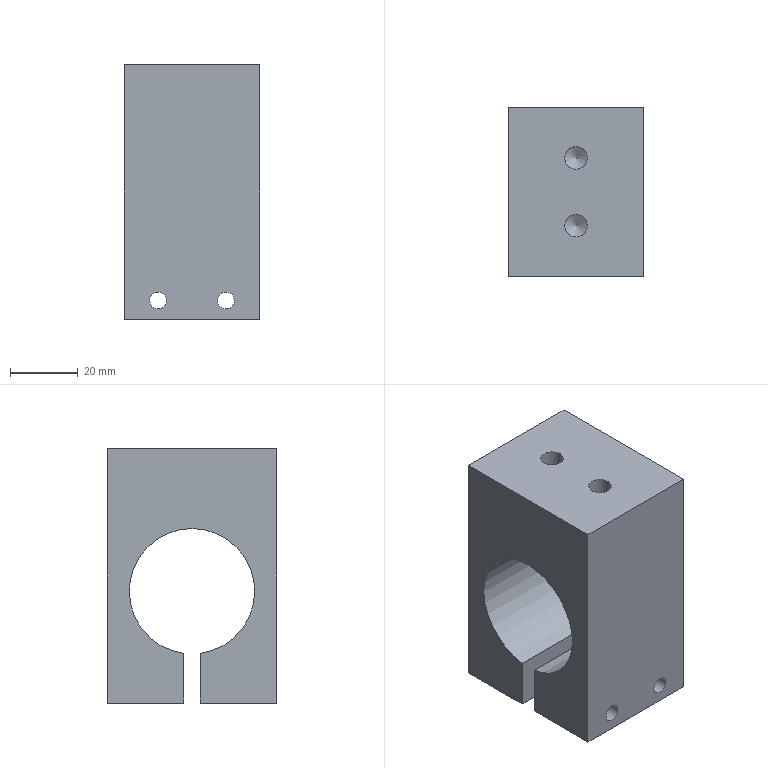Part | STEP file | SN10_010_003_SUPORTE | 1 solid | 18 faces | box 40 x 50 x 75 mm | volume 100062 mm3 | plane 9 | cylinder 7 | cone 2 | commonest cylinder face diameters 4.917 x2 6.647 x2 7 x2 37 x1
STEP:
#1=CARTESIAN_POINT('',(0.,0.,0.));
#2=DIRECTION('',(0.,0.,1.));
#3=DIRECTION('',(1.,0.,0.));
#4=AXIS2_PLACEMENT_3D('',#1,#2,#3);
#5=CARTESIAN_POINT('',(-7.842,117.5,231.679));
#6=VERTEX_POINT('',#5);
#7=CARTESIAN_POINT('',(-10.,117.5,230.5));
#8=DIRECTION('',(0.,1.,0.));
#9=DIRECTION('',(1.,0.,0.));
#10=AXIS2_PLACEMENT_3D('',#7,#8,#9);
#11=CIRCLE('',#10,2.458);
#12=CARTESIAN_POINT('',(-10.,117.4,230.5));
#13=DIRECTION('',(0.,-1.,0.));
#14=DIRECTION('',(0.8776,0.,0.4794));
#15=AXIS2_PLACEMENT_3D('',#12,#13,#14);
#16=CYLINDRICAL_SURFACE('',#15,2.458);
#17=CARTESIAN_POINT('',(12.066,-0.1));
#18=DIRECTION('',(-1.,0.));
#19=VECTOR('',#18,1.);
#20=LINE('',#17,#19);
#21=(GEOMETRIC_REPRESENTATION_CONTEXT(2)PARAMETRIC_REPRESENTATION_CONTEXT()REPRESENTATION_CONTEXT('',''));
#22=DEFINITIONAL_REPRESENTATION('',(#20),#21);
#23=PCURVE('',#16,#22);
#24=CARTESIAN_POINT('',(20.,117.5,239.67));
#25=DIRECTION('',(0.,1.,0.));
#26=DIRECTION('',(0.,0.,1.));
#27=AXIS2_PLACEMENT_3D('',#24,#25,#26);
#28=PLANE('',#27);
#29=CARTESIAN_POINT('',(-9.17,-30.));
#30=DIRECTION('',(0.,1.));
#31=AXIS2_PLACEMENT_2D('',#29,#30);
#32=CIRCLE('',#31,2.458);
#33=(GEOMETRIC_REPRESENTATION_CONTEXT(2)PARAMETRIC_REPRESENTATION_CONTEXT()REPRESENTATION_CONTEXT('',''));
#34=DEFINITIONAL_REPRESENTATION('',(#32),#33);
#35=PCURVE('',#28,#34);
#36=SURFACE_CURVE('',#11,(#23,#35),.PCURVE_S1.);
#37=EDGE_CURVE('',#6,#6,#36,.T.);
#38=ORIENTED_EDGE('',*,*,#37,.F.);
#39=CARTESIAN_POINT('',(-7.842,95.,231.679));
#40=VERTEX_POINT('',#39);
#41=CARTESIAN_POINT('',(-7.842,117.5,231.679));
#42=CARTESIAN_POINT('',(-7.842,95.,231.679));
#43=B_SPLINE_CURVE_WITH_KNOTS('',1,(#41,#42),.UNSPECIFIED.,.F.,.F.,(2,2),(-0.1,22.4),.PIECEWISE_BEZIER_KNOTS.);
#44=CARTESIAN_POINT('',(6.283,0.));
#45=DIRECTION('',(0.,1.));
#46=VECTOR('',#45,1.);
#47=LINE('',#44,#46);
#48=(GEOMETRIC_REPRESENTATION_CONTEXT(2)PARAMETRIC_REPRESENTATION_CONTEXT()REPRESENTATION_CONTEXT('',''));
#49=DEFINITIONAL_REPRESENTATION('',(#47),#48);
#50=PCURVE('',#16,#49);
#51=CARTESIAN_POINT('',(0.,0.));
#52=DIRECTION('',(0.,1.));
#53=VECTOR('',#52,1.);
#54=LINE('',#51,#53);
#55=(GEOMETRIC_REPRESENTATION_CONTEXT(2)PARAMETRIC_REPRESENTATION_CONTEXT()REPRESENTATION_CONTEXT('',''));
#56=DEFINITIONAL_REPRESENTATION('',(#54),#55);
#57=PCURVE('',#16,#56);
#58=SEAM_CURVE('',#43,(#50,#57),.PCURVE_S1.);
#59=EDGE_CURVE('',#6,#40,#58,.T.);
#60=ORIENTED_EDGE('',*,*,#59,.T.);
#61=CARTESIAN_POINT('',(-10.,95.,230.5));
#62=DIRECTION('',(0.,-1.,0.));
#63=DIRECTION('',(1.,0.,0.));
#64=AXIS2_PLACEMENT_3D('',#61,#62,#63);
#65=CIRCLE('',#64,2.458);
#66=CARTESIAN_POINT('',(-0.5,22.4));
#67=DIRECTION('',(1.,0.));
#68=VECTOR('',#67,1.);
#69=LINE('',#66,#68);
#70=(GEOMETRIC_REPRESENTATION_CONTEXT(2)PARAMETRIC_REPRESENTATION_CONTEXT()REPRESENTATION_CONTEXT('',''));
#71=DEFINITIONAL_REPRESENTATION('',(#69),#70);
#72=PCURVE('',#16,#71);
#73=CARTESIAN_POINT('',(0.,95.,300.));
#74=DIRECTION('',(0.,-1.,0.));
#75=DIRECTION('',(0.,0.,-1.));
#76=AXIS2_PLACEMENT_3D('',#73,#74,#75);
#77=PLANE('',#76);
#78=CARTESIAN_POINT('',(69.5,-10.));
#79=DIRECTION('',(0.,1.));
#80=AXIS2_PLACEMENT_2D('',#78,#79);
#81=CIRCLE('',#80,2.458);
#82=(GEOMETRIC_REPRESENTATION_CONTEXT(2)PARAMETRIC_REPRESENTATION_CONTEXT()REPRESENTATION_CONTEXT('',''));
#83=DEFINITIONAL_REPRESENTATION('',(#81),#82);
#84=PCURVE('',#77,#83);
#85=SURFACE_CURVE('',#65,(#72,#84),.PCURVE_S1.);
#86=EDGE_CURVE('',#40,#40,#85,.T.);
#87=ORIENTED_EDGE('',*,*,#86,.F.);
#88=ORIENTED_EDGE('',*,*,#59,.F.);
#89=EDGE_LOOP('',(#38,#60,#87,#88));
#90=FACE_BOUND('',#89,.F.);
#91=ADVANCED_FACE('',(#90),#16,.F.);
#92=CARTESIAN_POINT('',(20.,117.5,239.67));
#93=VERTEX_POINT('',#92);
#94=CARTESIAN_POINT('',(-20.,117.5,239.67));
#95=VERTEX_POINT('',#94);
#96=CARTESIAN_POINT('',(20.,117.5,239.67));
#97=DIRECTION('',(-1.,0.,0.));
#98=VECTOR('',#97,1.);
#99=LINE('',#96,#98);
#100=CARTESIAN_POINT('',(0.,0.));
#101=DIRECTION('',(0.,-1.));
#102=VECTOR('',#101,1.);
#103=LINE('',#100,#102);
#104=(GEOMETRIC_REPRESENTATION_CONTEXT(2)PARAMETRIC_REPRESENTATION_CONTEXT()REPRESENTATION_CONTEXT('',''));
#105=DEFINITIONAL_REPRESENTATION('',(#103),#104);
#106=PCURVE('',#28,#105);
#107=CARTESIAN_POINT('',(19.9,120.,258.));
#108=DIRECTION('',(-1.,0.,0.));
#109=DIRECTION('',(0.,0.8776,-0.4794));
#110=AXIS2_PLACEMENT_3D('',#107,#108,#109);
#111=CYLINDRICAL_SURFACE('',#110,18.5);
#112=CARTESIAN_POINT('',(1.206,-0.1));
#113=DIRECTION('',(0.,1.));
#114=VECTOR('',#113,1.);
#115=LINE('',#112,#114);
#116=(GEOMETRIC_REPRESENTATION_CONTEXT(2)PARAMETRIC_REPRESENTATION_CONTEXT()REPRESENTATION_CONTEXT('',''));
#117=DEFINITIONAL_REPRESENTATION('',(#115),#116);
#118=PCURVE('',#111,#117);
#119=SURFACE_CURVE('',#99,(#106,#118),.PCURVE_S1.);
#120=EDGE_CURVE('',#93,#95,#119,.T.);
#121=ORIENTED_EDGE('',*,*,#120,.F.);
#122=CARTESIAN_POINT('',(20.,117.5,225.));
#123=VERTEX_POINT('',#122);
#124=CARTESIAN_POINT('',(20.,117.5,239.67));
#125=DIRECTION('',(0.,0.,-1.));
#126=VECTOR('',#125,1.);
#127=LINE('',#124,#126);
#128=CARTESIAN_POINT('',(0.,0.));
#129=DIRECTION('',(-1.,0.));
#130=VECTOR('',#129,1.);
#131=LINE('',#128,#130);
#132=(GEOMETRIC_REPRESENTATION_CONTEXT(2)PARAMETRIC_REPRESENTATION_CONTEXT()REPRESENTATION_CONTEXT('',''));
#133=DEFINITIONAL_REPRESENTATION('',(#131),#132);
#134=PCURVE('',#28,#133);
#135=CARTESIAN_POINT('',(20.,120.,300.));
#136=DIRECTION('',(1.,0.,0.));
#137=DIRECTION('',(0.,0.,-1.));
#138=AXIS2_PLACEMENT_3D('',#135,#136,#137);
#139=PLANE('',#138);
#140=CARTESIAN_POINT('',(60.33,-2.5));
#141=DIRECTION('',(1.,0.));
#142=VECTOR('',#141,1.);
#143=LINE('',#140,#142);
#144=(GEOMETRIC_REPRESENTATION_CONTEXT(2)PARAMETRIC_REPRESENTATION_CONTEXT()REPRESENTATION_CONTEXT('',''));
#145=DEFINITIONAL_REPRESENTATION('',(#143),#144);
#146=PCURVE('',#139,#145);
#147=SURFACE_CURVE('',#127,(#134,#146),.PCURVE_S1.);
#148=EDGE_CURVE('',#93,#123,#147,.T.);
#149=ORIENTED_EDGE('',*,*,#148,.T.);
#150=CARTESIAN_POINT('',(-20.,117.5,225.));
#151=VERTEX_POINT('',#150);
#152=CARTESIAN_POINT('',(20.,117.5,225.));
#153=DIRECTION('',(-1.,0.,0.));
#154=VECTOR('',#153,1.);
#155=LINE('',#152,#154);
#156=CARTESIAN_POINT('',(-14.67,0.));
#157=DIRECTION('',(0.,-1.));
#158=VECTOR('',#157,1.);
#159=LINE('',#156,#158);
#160=(GEOMETRIC_REPRESENTATION_CONTEXT(2)PARAMETRIC_REPRESENTATION_CONTEXT()REPRESENTATION_CONTEXT('',''));
#161=DEFINITIONAL_REPRESENTATION('',(#159),#160);
#162=PCURVE('',#28,#161);
#163=CARTESIAN_POINT('',(0.,145.,225.));
#164=DIRECTION('',(0.,0.,1.));
#165=DIRECTION('',(1.,0.,0.));
#166=AXIS2_PLACEMENT_3D('',#163,#164,#165);
#167=PLANE('',#166);
#168=CARTESIAN_POINT('',(20.,-27.5));
#169=DIRECTION('',(-1.,0.));
#170=VECTOR('',#169,1.);
#171=LINE('',#168,#170);
#172=(GEOMETRIC_REPRESENTATION_CONTEXT(2)PARAMETRIC_REPRESENTATION_CONTEXT()REPRESENTATION_CONTEXT('',''));
#173=DEFINITIONAL_REPRESENTATION('',(#171),#172);
#174=PCURVE('',#167,#173);
#175=SURFACE_CURVE('',#155,(#162,#174),.PCURVE_S1.);
#176=EDGE_CURVE('',#123,#151,#175,.T.);
#177=ORIENTED_EDGE('',*,*,#176,.T.);
#178=CARTESIAN_POINT('',(-20.,117.5,225.));
#179=DIRECTION('',(0.,0.,1.));
#180=VECTOR('',#179,1.);
#181=LINE('',#178,#180);
#182=CARTESIAN_POINT('',(-14.67,-40.));
#183=DIRECTION('',(1.,0.));
#184=VECTOR('',#183,1.);
#185=LINE('',#182,#184);
#186=(GEOMETRIC_REPRESENTATION_CONTEXT(2)PARAMETRIC_REPRESENTATION_CONTEXT()REPRESENTATION_CONTEXT('',''));
#187=DEFINITIONAL_REPRESENTATION('',(#185),#186);
#188=PCURVE('',#28,#187);
#189=CARTESIAN_POINT('',(-20.,120.,300.));
#190=DIRECTION('',(1.,0.,0.));
#191=DIRECTION('',(0.,0.,-1.));
#192=AXIS2_PLACEMENT_3D('',#189,#190,#191);
#193=PLANE('',#192);
#194=CARTESIAN_POINT('',(75.,-2.5));
#195=DIRECTION('',(-1.,0.));
#196=VECTOR('',#195,1.);
#197=LINE('',#194,#196);
#198=(GEOMETRIC_REPRESENTATION_CONTEXT(2)PARAMETRIC_REPRESENTATION_CONTEXT()REPRESENTATION_CONTEXT('',''));
#199=DEFINITIONAL_REPRESENTATION('',(#197),#198);
#200=PCURVE('',#193,#199);
#201=SURFACE_CURVE('',#181,(#188,#200),.PCURVE_S1.);
#202=EDGE_CURVE('',#151,#95,#201,.T.);
#203=ORIENTED_EDGE('',*,*,#202,.T.);
#204=EDGE_LOOP('',(#121,#149,#177,#203));
#205=FACE_BOUND('',#204,.T.);
#206=ORIENTED_EDGE('',*,*,#37,.F.);
#207=EDGE_LOOP('',(#206));
#208=FACE_BOUND('',#207,.T.);
#209=CARTESIAN_POINT('',(12.158,117.5,231.679));
#210=VERTEX_POINT('',#209);
#211=CARTESIAN_POINT('',(10.,117.5,230.5));
#212=DIRECTION('',(0.,1.,0.));
#213=DIRECTION('',(1.,0.,0.));
#214=AXIS2_PLACEMENT_3D('',#211,#212,#213);
#215=CIRCLE('',#214,2.458);
#216=CARTESIAN_POINT('',(-9.17,-10.));
#217=DIRECTION('',(0.,1.));
#218=AXIS2_PLACEMENT_2D('',#216,#217);
#219=CIRCLE('',#218,2.458);
#220=(GEOMETRIC_REPRESENTATION_CONTEXT(2)PARAMETRIC_REPRESENTATION_CONTEXT()REPRESENTATION_CONTEXT('',''));
#221=DEFINITIONAL_REPRESENTATION('',(#219),#220);
#222=PCURVE('',#28,#221);
#223=CARTESIAN_POINT('',(10.,117.4,230.5));
#224=DIRECTION('',(0.,-1.,0.));
#225=DIRECTION('',(0.8776,0.,0.4794));
#226=AXIS2_PLACEMENT_3D('',#223,#224,#225);
#227=CYLINDRICAL_SURFACE('',#226,2.458);
#228=CARTESIAN_POINT('',(12.066,-0.1));
#229=DIRECTION('',(-1.,0.));
#230=VECTOR('',#229,1.);
#231=LINE('',#228,#230);
#232=(GEOMETRIC_REPRESENTATION_CONTEXT(2)PARAMETRIC_REPRESENTATION_CONTEXT()REPRESENTATION_CONTEXT('',''));
#233=DEFINITIONAL_REPRESENTATION('',(#231),#232);
#234=PCURVE('',#227,#233);
#235=SURFACE_CURVE('',#215,(#222,#234),.PCURVE_S1.);
#236=EDGE_CURVE('',#210,#210,#235,.T.);
#237=ORIENTED_EDGE('',*,*,#236,.F.);
#238=EDGE_LOOP('',(#237));
#239=FACE_BOUND('',#238,.T.);
#240=ADVANCED_FACE('',(#205,#208,#239),#28,.T.);
#241=CARTESIAN_POINT('',(-20.,95.,300.));
#242=VERTEX_POINT('',#241);
#243=CARTESIAN_POINT('',(20.,95.,300.));
#244=VERTEX_POINT('',#243);
#245=CARTESIAN_POINT('',(-20.,95.,300.));
#246=DIRECTION('',(1.,0.,0.));
#247=VECTOR('',#246,1.);
#248=LINE('',#245,#247);
#249=CARTESIAN_POINT('',(0.,-20.));
#250=DIRECTION('',(0.,1.));
#251=VECTOR('',#250,1.);
#252=LINE('',#249,#251);
#253=(GEOMETRIC_REPRESENTATION_CONTEXT(2)PARAMETRIC_REPRESENTATION_CONTEXT()REPRESENTATION_CONTEXT('',''));
#254=DEFINITIONAL_REPRESENTATION('',(#252),#253);
#255=PCURVE('',#77,#254);
#256=CARTESIAN_POINT('',(0.,95.,300.));
#257=DIRECTION('',(0.,0.,-1.));
#258=DIRECTION('',(-1.,0.,0.));
#259=AXIS2_PLACEMENT_3D('',#256,#257,#258);
#260=PLANE('',#259);
#261=CARTESIAN_POINT('',(20.,0.));
#262=DIRECTION('',(-1.,0.));
#263=VECTOR('',#262,1.);
#264=LINE('',#261,#263);
#265=(GEOMETRIC_REPRESENTATION_CONTEXT(2)PARAMETRIC_REPRESENTATION_CONTEXT()REPRESENTATION_CONTEXT('',''));
#266=DEFINITIONAL_REPRESENTATION('',(#264),#265);
#267=PCURVE('',#260,#266);
#268=SURFACE_CURVE('',#248,(#255,#267),.PCURVE_S1.);
#269=EDGE_CURVE('',#242,#244,#268,.T.);
#270=ORIENTED_EDGE('',*,*,#269,.F.);
#271=CARTESIAN_POINT('',(-20.,95.,225.));
#272=VERTEX_POINT('',#271);
#273=CARTESIAN_POINT('',(-20.,95.,300.));
#274=DIRECTION('',(0.,0.,-1.));
#275=VECTOR('',#274,1.);
#276=LINE('',#273,#275);
#277=CARTESIAN_POINT('',(0.,-20.));
#278=DIRECTION('',(1.,0.));
#279=VECTOR('',#278,1.);
#280=LINE('',#277,#279);
#281=(GEOMETRIC_REPRESENTATION_CONTEXT(2)PARAMETRIC_REPRESENTATION_CONTEXT()REPRESENTATION_CONTEXT('',''));
#282=DEFINITIONAL_REPRESENTATION('',(#280),#281);
#283=PCURVE('',#77,#282);
#284=CARTESIAN_POINT('',(0.,-25.));
#285=DIRECTION('',(1.,0.));
#286=VECTOR('',#285,1.);
#287=LINE('',#284,#286);
#288=(GEOMETRIC_REPRESENTATION_CONTEXT(2)PARAMETRIC_REPRESENTATION_CONTEXT()REPRESENTATION_CONTEXT('',''));
#289=DEFINITIONAL_REPRESENTATION('',(#287),#288);
#290=PCURVE('',#193,#289);
#291=SURFACE_CURVE('',#276,(#283,#290),.PCURVE_S1.);
#292=EDGE_CURVE('',#242,#272,#291,.T.);
#293=ORIENTED_EDGE('',*,*,#292,.T.);
#294=CARTESIAN_POINT('',(20.,95.,225.));
#295=VERTEX_POINT('',#294);
#296=CARTESIAN_POINT('',(-20.,95.,225.));
#297=DIRECTION('',(1.,0.,0.));
#298=VECTOR('',#297,1.);
#299=LINE('',#296,#298);
#300=CARTESIAN_POINT('',(75.,-20.));
#301=DIRECTION('',(0.,1.));
#302=VECTOR('',#301,1.);
#303=LINE('',#300,#302);
#304=(GEOMETRIC_REPRESENTATION_CONTEXT(2)PARAMETRIC_REPRESENTATION_CONTEXT()REPRESENTATION_CONTEXT('',''));
#305=DEFINITIONAL_REPRESENTATION('',(#303),#304);
#306=PCURVE('',#77,#305);
#307=CARTESIAN_POINT('',(-20.,-50.));
#308=DIRECTION('',(1.,0.));
#309=VECTOR('',#308,1.);
#310=LINE('',#307,#309);
#311=(GEOMETRIC_REPRESENTATION_CONTEXT(2)PARAMETRIC_REPRESENTATION_CONTEXT()REPRESENTATION_CONTEXT('',''));
#312=DEFINITIONAL_REPRESENTATION('',(#310),#311);
#313=PCURVE('',#167,#312);
#314=SURFACE_CURVE('',#299,(#306,#313),.PCURVE_S1.);
#315=EDGE_CURVE('',#272,#295,#314,.T.);
#316=ORIENTED_EDGE('',*,*,#315,.T.);
#317=CARTESIAN_POINT('',(20.,95.,300.));
#318=DIRECTION('',(0.,0.,-1.));
#319=VECTOR('',#318,1.);
#320=LINE('',#317,#319);
#321=CARTESIAN_POINT('',(0.,20.));
#322=DIRECTION('',(1.,0.));
#323=VECTOR('',#322,1.);
#324=LINE('',#321,#323);
#325=(GEOMETRIC_REPRESENTATION_CONTEXT(2)PARAMETRIC_REPRESENTATION_CONTEXT()REPRESENTATION_CONTEXT('',''));
#326=DEFINITIONAL_REPRESENTATION('',(#324),#325);
#327=PCURVE('',#77,#326);
#328=CARTESIAN_POINT('',(0.,-25.));
#329=DIRECTION('',(1.,0.));
#330=VECTOR('',#329,1.);
#331=LINE('',#328,#330);
#332=(GEOMETRIC_REPRESENTATION_CONTEXT(2)PARAMETRIC_REPRESENTATION_CONTEXT()REPRESENTATION_CONTEXT('',''));
#333=DEFINITIONAL_REPRESENTATION('',(#331),#332);
#334=PCURVE('',#139,#333);
#335=SURFACE_CURVE('',#320,(#327,#334),.PCURVE_S1.);
#336=EDGE_CURVE('',#244,#295,#335,.T.);
#337=ORIENTED_EDGE('',*,*,#336,.F.);
#338=EDGE_LOOP('',(#270,#293,#316,#337));
#339=FACE_BOUND('',#338,.T.);
#340=ORIENTED_EDGE('',*,*,#86,.F.);
#341=EDGE_LOOP('',(#340));
#342=FACE_BOUND('',#341,.T.);
#343=CARTESIAN_POINT('',(12.158,95.,231.679));
#344=VERTEX_POINT('',#343);
#345=CARTESIAN_POINT('',(10.,95.,230.5));
#346=DIRECTION('',(0.,-1.,0.));
#347=DIRECTION('',(1.,0.,0.));
#348=AXIS2_PLACEMENT_3D('',#345,#346,#347);
#349=CIRCLE('',#348,2.458);
#350=CARTESIAN_POINT('',(69.5,10.));
#351=DIRECTION('',(0.,1.));
#352=AXIS2_PLACEMENT_2D('',#350,#351);
#353=CIRCLE('',#352,2.458);
#354=(GEOMETRIC_REPRESENTATION_CONTEXT(2)PARAMETRIC_REPRESENTATION_CONTEXT()REPRESENTATION_CONTEXT('',''));
#355=DEFINITIONAL_REPRESENTATION('',(#353),#354);
#356=PCURVE('',#77,#355);
#357=CARTESIAN_POINT('',(-0.5,22.4));
#358=DIRECTION('',(1.,0.));
#359=VECTOR('',#358,1.);
#360=LINE('',#357,#359);
#361=(GEOMETRIC_REPRESENTATION_CONTEXT(2)PARAMETRIC_REPRESENTATION_CONTEXT()REPRESENTATION_CONTEXT('',''));
#362=DEFINITIONAL_REPRESENTATION('',(#360),#361);
#363=PCURVE('',#227,#362);
#364=SURFACE_CURVE('',#349,(#356,#363),.PCURVE_S1.);
#365=EDGE_CURVE('',#344,#344,#364,.T.);
#366=ORIENTED_EDGE('',*,*,#365,.F.);
#367=EDGE_LOOP('',(#366));
#368=FACE_BOUND('',#367,.T.);
#369=ADVANCED_FACE('',(#339,#342,#368),#77,.T.);
#370=CARTESIAN_POINT('',(20.,145.,225.));
#371=VERTEX_POINT('',#370);
#372=CARTESIAN_POINT('',(20.,122.5,225.));
#373=VERTEX_POINT('',#372);
#374=CARTESIAN_POINT('',(20.,145.,225.));
#375=DIRECTION('',(0.,-1.,0.));
#376=VECTOR('',#375,1.);
#377=LINE('',#374,#376);
#378=CARTESIAN_POINT('',(75.,25.));
#379=DIRECTION('',(0.,-1.));
#380=VECTOR('',#379,1.);
#381=LINE('',#378,#380);
#382=(GEOMETRIC_REPRESENTATION_CONTEXT(2)PARAMETRIC_REPRESENTATION_CONTEXT()REPRESENTATION_CONTEXT('',''));
#383=DEFINITIONAL_REPRESENTATION('',(#381),#382);
#384=PCURVE('',#139,#383);
#385=CARTESIAN_POINT('',(0.,145.,225.));
#386=DIRECTION('',(0.,0.,1.));
#387=DIRECTION('',(1.,0.,0.));
#388=AXIS2_PLACEMENT_3D('',#385,#386,#387);
#389=PLANE('',#388);
#390=CARTESIAN_POINT('',(20.,0.));
#391=DIRECTION('',(0.,-1.));
#392=VECTOR('',#391,1.);
#393=LINE('',#390,#392);
#394=(GEOMETRIC_REPRESENTATION_CONTEXT(2)PARAMETRIC_REPRESENTATION_CONTEXT()REPRESENTATION_CONTEXT('',''));
#395=DEFINITIONAL_REPRESENTATION('',(#393),#394);
#396=PCURVE('',#389,#395);
#397=SURFACE_CURVE('',#377,(#384,#396),.PCURVE_S1.);
#398=EDGE_CURVE('',#371,#373,#397,.T.);
#399=ORIENTED_EDGE('',*,*,#398,.F.);
#400=CARTESIAN_POINT('',(20.,145.,300.));
#401=VERTEX_POINT('',#400);
#402=CARTESIAN_POINT('',(20.,145.,225.));
#403=DIRECTION('',(0.,0.,1.));
#404=VECTOR('',#403,1.);
#405=LINE('',#402,#404);
#406=CARTESIAN_POINT('',(75.,25.));
#407=DIRECTION('',(-1.,0.));
#408=VECTOR('',#407,1.);
#409=LINE('',#406,#408);
#410=(GEOMETRIC_REPRESENTATION_CONTEXT(2)PARAMETRIC_REPRESENTATION_CONTEXT()REPRESENTATION_CONTEXT('',''));
#411=DEFINITIONAL_REPRESENTATION('',(#409),#410);
#412=PCURVE('',#139,#411);
#413=CARTESIAN_POINT('',(0.,145.,225.));
#414=DIRECTION('',(0.,1.,0.));
#415=DIRECTION('',(0.,0.,1.));
#416=AXIS2_PLACEMENT_3D('',#413,#414,#415);
#417=PLANE('',#416);
#418=CARTESIAN_POINT('',(0.,20.));
#419=DIRECTION('',(1.,0.));
#420=VECTOR('',#419,1.);
#421=LINE('',#418,#420);
#422=(GEOMETRIC_REPRESENTATION_CONTEXT(2)PARAMETRIC_REPRESENTATION_CONTEXT()REPRESENTATION_CONTEXT('',''));
#423=DEFINITIONAL_REPRESENTATION('',(#421),#422);
#424=PCURVE('',#417,#423);
#425=SURFACE_CURVE('',#405,(#412,#424),.PCURVE_S1.);
#426=EDGE_CURVE('',#371,#401,#425,.T.);
#427=ORIENTED_EDGE('',*,*,#426,.T.);
#428=CARTESIAN_POINT('',(20.,95.,300.));
#429=DIRECTION('',(0.,1.,0.));
#430=VECTOR('',#429,1.);
#431=LINE('',#428,#430);
#432=CARTESIAN_POINT('',(0.,-25.));
#433=DIRECTION('',(0.,1.));
#434=VECTOR('',#433,1.);
#435=LINE('',#432,#434);
#436=(GEOMETRIC_REPRESENTATION_CONTEXT(2)PARAMETRIC_REPRESENTATION_CONTEXT()REPRESENTATION_CONTEXT('',''));
#437=DEFINITIONAL_REPRESENTATION('',(#435),#436);
#438=PCURVE('',#139,#437);
#439=CARTESIAN_POINT('',(-20.,0.));
#440=DIRECTION('',(0.,1.));
#441=VECTOR('',#440,1.);
#442=LINE('',#439,#441);
#443=(GEOMETRIC_REPRESENTATION_CONTEXT(2)PARAMETRIC_REPRESENTATION_CONTEXT()REPRESENTATION_CONTEXT('',''));
#444=DEFINITIONAL_REPRESENTATION('',(#442),#443);
#445=PCURVE('',#260,#444);
#446=SURFACE_CURVE('',#431,(#438,#445),.PCURVE_S1.);
#447=EDGE_CURVE('',#244,#401,#446,.T.);
#448=ORIENTED_EDGE('',*,*,#447,.F.);
#449=ORIENTED_EDGE('',*,*,#336,.T.);
#450=CARTESIAN_POINT('',(20.,117.5,225.));
#451=DIRECTION('',(0.,-1.,0.));
#452=VECTOR('',#451,1.);
#453=LINE('',#450,#452);
#454=CARTESIAN_POINT('',(75.,-2.5));
#455=DIRECTION('',(0.,-1.));
#456=VECTOR('',#455,1.);
#457=LINE('',#454,#456);
#458=(GEOMETRIC_REPRESENTATION_CONTEXT(2)PARAMETRIC_REPRESENTATION_CONTEXT()REPRESENTATION_CONTEXT('',''));
#459=DEFINITIONAL_REPRESENTATION('',(#457),#458);
#460=PCURVE('',#139,#459);
#461=CARTESIAN_POINT('',(20.,-27.5));
#462=DIRECTION('',(0.,-1.));
#463=VECTOR('',#462,1.);
#464=LINE('',#461,#463);
#465=(GEOMETRIC_REPRESENTATION_CONTEXT(2)PARAMETRIC_REPRESENTATION_CONTEXT()REPRESENTATION_CONTEXT('',''));
#466=DEFINITIONAL_REPRESENTATION('',(#464),#465);
#467=PCURVE('',#167,#466);
#468=SURFACE_CURVE('',#453,(#460,#467),.PCURVE_S1.);
#469=EDGE_CURVE('',#123,#295,#468,.T.);
#470=ORIENTED_EDGE('',*,*,#469,.F.);
#471=ORIENTED_EDGE('',*,*,#148,.F.);
#472=CARTESIAN_POINT('',(20.,122.5,239.67));
#473=VERTEX_POINT('',#472);
#474=CARTESIAN_POINT('',(20.,120.,258.));
#475=DIRECTION('',(1.,0.,0.));
#476=DIRECTION('',(0.,1.,0.));
#477=AXIS2_PLACEMENT_3D('',#474,#475,#476);
#478=CIRCLE('',#477,18.5);
#479=CARTESIAN_POINT('',(42.,0.));
#480=DIRECTION('',(0.,1.));
#481=AXIS2_PLACEMENT_2D('',#479,#480);
#482=CIRCLE('',#481,18.5);
#483=(GEOMETRIC_REPRESENTATION_CONTEXT(2)PARAMETRIC_REPRESENTATION_CONTEXT()REPRESENTATION_CONTEXT('',''));
#484=DEFINITIONAL_REPRESENTATION('',(#482),#483);
#485=PCURVE('',#139,#484);
#486=CARTESIAN_POINT('',(12.066,-0.1));
#487=DIRECTION('',(-1.,0.));
#488=VECTOR('',#487,1.);
#489=LINE('',#486,#488);
#490=(GEOMETRIC_REPRESENTATION_CONTEXT(2)PARAMETRIC_REPRESENTATION_CONTEXT()REPRESENTATION_CONTEXT('',''));
#491=DEFINITIONAL_REPRESENTATION('',(#489),#490);
#492=PCURVE('',#111,#491);
#493=SURFACE_CURVE('',#478,(#485,#492),.PCURVE_S1.);
#494=EDGE_CURVE('',#473,#93,#493,.T.);
#495=ORIENTED_EDGE('',*,*,#494,.F.);
#496=CARTESIAN_POINT('',(20.,122.5,225.));
#497=DIRECTION('',(0.,0.,1.));
#498=VECTOR('',#497,1.);
#499=LINE('',#496,#498);
#500=CARTESIAN_POINT('',(75.,2.5));
#501=DIRECTION('',(-1.,0.));
#502=VECTOR('',#501,1.);
#503=LINE('',#500,#502);
#504=(GEOMETRIC_REPRESENTATION_CONTEXT(2)PARAMETRIC_REPRESENTATION_CONTEXT()REPRESENTATION_CONTEXT('',''));
#505=DEFINITIONAL_REPRESENTATION('',(#503),#504);
#506=PCURVE('',#139,#505);
#507=CARTESIAN_POINT('',(20.,122.5,225.));
#508=DIRECTION('',(0.,-1.,0.));
#509=DIRECTION('',(0.,0.,-1.));
#510=AXIS2_PLACEMENT_3D('',#507,#508,#509);
#511=PLANE('',#510);
#512=CARTESIAN_POINT('',(0.,0.));
#513=DIRECTION('',(-1.,0.));
#514=VECTOR('',#513,1.);
#515=LINE('',#512,#514);
#516=(GEOMETRIC_REPRESENTATION_CONTEXT(2)PARAMETRIC_REPRESENTATION_CONTEXT()REPRESENTATION_CONTEXT('',''));
#517=DEFINITIONAL_REPRESENTATION('',(#515),#516);
#518=PCURVE('',#511,#517);
#519=SURFACE_CURVE('',#499,(#506,#518),.PCURVE_S1.);
#520=EDGE_CURVE('',#373,#473,#519,.T.);
#521=ORIENTED_EDGE('',*,*,#520,.F.);
#522=EDGE_LOOP('',(#399,#427,#448,#449,#470,#471,#495,#521));
#523=FACE_BOUND('',#522,.T.);
#524=ADVANCED_FACE('',(#523),#139,.T.);
#525=ORIENTED_EDGE('',*,*,#176,.F.);
#526=ORIENTED_EDGE('',*,*,#469,.T.);
#527=ORIENTED_EDGE('',*,*,#315,.F.);
#528=CARTESIAN_POINT('',(-20.,117.5,225.));
#529=DIRECTION('',(0.,-1.,0.));
#530=VECTOR('',#529,1.);
#531=LINE('',#528,#530);
#532=CARTESIAN_POINT('',(-20.,-27.5));
#533=DIRECTION('',(0.,-1.));
#534=VECTOR('',#533,1.);
#535=LINE('',#532,#534);
#536=(GEOMETRIC_REPRESENTATION_CONTEXT(2)PARAMETRIC_REPRESENTATION_CONTEXT()REPRESENTATION_CONTEXT('',''));
#537=DEFINITIONAL_REPRESENTATION('',(#535),#536);
#538=PCURVE('',#167,#537);
#539=CARTESIAN_POINT('',(75.,-2.5));
#540=DIRECTION('',(0.,-1.));
#541=VECTOR('',#540,1.);
#542=LINE('',#539,#541);
#543=(GEOMETRIC_REPRESENTATION_CONTEXT(2)PARAMETRIC_REPRESENTATION_CONTEXT()REPRESENTATION_CONTEXT('',''));
#544=DEFINITIONAL_REPRESENTATION('',(#542),#543);
#545=PCURVE('',#193,#544);
#546=SURFACE_CURVE('',#531,(#538,#545),.PCURVE_S1.);
#547=EDGE_CURVE('',#151,#272,#546,.T.);
#548=ORIENTED_EDGE('',*,*,#547,.F.);
#549=EDGE_LOOP('',(#525,#526,#527,#548));
#550=FACE_BOUND('',#549,.T.);
#551=ADVANCED_FACE('',(#550),#167,.F.);
#552=CARTESIAN_POINT('',(-20.,122.5,225.));
#553=VERTEX_POINT('',#552);
#554=CARTESIAN_POINT('',(-20.,122.5,239.67));
#555=VERTEX_POINT('',#554);
#556=CARTESIAN_POINT('',(-20.,122.5,225.));
#557=DIRECTION('',(0.,0.,1.));
#558=VECTOR('',#557,1.);
#559=LINE('',#556,#558);
#560=CARTESIAN_POINT('',(75.,2.5));
#561=DIRECTION('',(-1.,0.));
#562=VECTOR('',#561,1.);
#563=LINE('',#560,#562);
#564=(GEOMETRIC_REPRESENTATION_CONTEXT(2)PARAMETRIC_REPRESENTATION_CONTEXT()REPRESENTATION_CONTEXT('',''));
#565=DEFINITIONAL_REPRESENTATION('',(#563),#564);
#566=PCURVE('',#193,#565);
#567=CARTESIAN_POINT('',(0.,-40.));
#568=DIRECTION('',(-1.,0.));
#569=VECTOR('',#568,1.);
#570=LINE('',#567,#569);
#571=(GEOMETRIC_REPRESENTATION_CONTEXT(2)PARAMETRIC_REPRESENTATION_CONTEXT()REPRESENTATION_CONTEXT('',''));
#572=DEFINITIONAL_REPRESENTATION('',(#570),#571);
#573=PCURVE('',#511,#572);
#574=SURFACE_CURVE('',#559,(#566,#573),.PCURVE_S1.);
#575=EDGE_CURVE('',#553,#555,#574,.T.);
#576=ORIENTED_EDGE('',*,*,#575,.T.);
#577=CARTESIAN_POINT('',(-20.,120.,258.));
#578=DIRECTION('',(1.,0.,0.));
#579=DIRECTION('',(0.,1.,0.));
#580=AXIS2_PLACEMENT_3D('',#577,#578,#579);
#581=CIRCLE('',#580,18.5);
#582=CARTESIAN_POINT('',(42.,0.));
#583=DIRECTION('',(0.,1.));
#584=AXIS2_PLACEMENT_2D('',#582,#583);
#585=CIRCLE('',#584,18.5);
#586=(GEOMETRIC_REPRESENTATION_CONTEXT(2)PARAMETRIC_REPRESENTATION_CONTEXT()REPRESENTATION_CONTEXT('',''));
#587=DEFINITIONAL_REPRESENTATION('',(#585),#586);
#588=PCURVE('',#193,#587);
#589=CARTESIAN_POINT('',(12.066,39.9));
#590=DIRECTION('',(-1.,0.));
#591=VECTOR('',#590,1.);
#592=LINE('',#589,#591);
#593=(GEOMETRIC_REPRESENTATION_CONTEXT(2)PARAMETRIC_REPRESENTATION_CONTEXT()REPRESENTATION_CONTEXT('',''));
#594=DEFINITIONAL_REPRESENTATION('',(#592),#593);
#595=PCURVE('',#111,#594);
#596=SURFACE_CURVE('',#581,(#588,#595),.PCURVE_S1.);
#597=EDGE_CURVE('',#555,#95,#596,.T.);
#598=ORIENTED_EDGE('',*,*,#597,.T.);
#599=ORIENTED_EDGE('',*,*,#202,.F.);
#600=ORIENTED_EDGE('',*,*,#547,.T.);
#601=ORIENTED_EDGE('',*,*,#292,.F.);
#602=CARTESIAN_POINT('',(-20.,145.,300.));
#603=VERTEX_POINT('',#602);
#604=CARTESIAN_POINT('',(-20.,95.,300.));
#605=DIRECTION('',(0.,1.,0.));
#606=VECTOR('',#605,1.);
#607=LINE('',#604,#606);
#608=CARTESIAN_POINT('',(0.,-25.));
#609=DIRECTION('',(0.,1.));
#610=VECTOR('',#609,1.);
#611=LINE('',#608,#610);
#612=(GEOMETRIC_REPRESENTATION_CONTEXT(2)PARAMETRIC_REPRESENTATION_CONTEXT()REPRESENTATION_CONTEXT('',''));
#613=DEFINITIONAL_REPRESENTATION('',(#611),#612);
#614=PCURVE('',#193,#613);
#615=CARTESIAN_POINT('',(20.,0.));
#616=DIRECTION('',(0.,1.));
#617=VECTOR('',#616,1.);
#618=LINE('',#615,#617);
#619=(GEOMETRIC_REPRESENTATION_CONTEXT(2)PARAMETRIC_REPRESENTATION_CONTEXT()REPRESENTATION_CONTEXT('',''));
#620=DEFINITIONAL_REPRESENTATION('',(#618),#619);
#621=PCURVE('',#260,#620);
#622=SURFACE_CURVE('',#607,(#614,#621),.PCURVE_S1.);
#623=EDGE_CURVE('',#242,#603,#622,.T.);
#624=ORIENTED_EDGE('',*,*,#623,.T.);
#625=CARTESIAN_POINT('',(-20.,145.,225.));
#626=VERTEX_POINT('',#625);
#627=CARTESIAN_POINT('',(-20.,145.,225.));
#628=DIRECTION('',(0.,0.,1.));
#629=VECTOR('',#628,1.);
#630=LINE('',#627,#629);
#631=CARTESIAN_POINT('',(75.,25.));
#632=DIRECTION('',(-1.,0.));
#633=VECTOR('',#632,1.);
#634=LINE('',#631,#633);
#635=(GEOMETRIC_REPRESENTATION_CONTEXT(2)PARAMETRIC_REPRESENTATION_CONTEXT()REPRESENTATION_CONTEXT('',''));
#636=DEFINITIONAL_REPRESENTATION('',(#634),#635);
#637=PCURVE('',#193,#636);
#638=CARTESIAN_POINT('',(0.,-20.));
#639=DIRECTION('',(1.,0.));
#640=VECTOR('',#639,1.);
#641=LINE('',#638,#640);
#642=(GEOMETRIC_REPRESENTATION_CONTEXT(2)PARAMETRIC_REPRESENTATION_CONTEXT()REPRESENTATION_CONTEXT('',''));
#643=DEFINITIONAL_REPRESENTATION('',(#641),#642);
#644=PCURVE('',#417,#643);
#645=SURFACE_CURVE('',#630,(#637,#644),.PCURVE_S1.);
#646=EDGE_CURVE('',#626,#603,#645,.T.);
#647=ORIENTED_EDGE('',*,*,#646,.F.);
#648=CARTESIAN_POINT('',(-20.,145.,225.));
#649=DIRECTION('',(0.,-1.,0.));
#650=VECTOR('',#649,1.);
#651=LINE('',#648,#650);
#652=CARTESIAN_POINT('',(75.,25.));
#653=DIRECTION('',(0.,-1.));
#654=VECTOR('',#653,1.);
#655=LINE('',#652,#654);
#656=(GEOMETRIC_REPRESENTATION_CONTEXT(2)PARAMETRIC_REPRESENTATION_CONTEXT()REPRESENTATION_CONTEXT('',''));
#657=DEFINITIONAL_REPRESENTATION('',(#655),#656);
#658=PCURVE('',#193,#657);
#659=CARTESIAN_POINT('',(-20.,0.));
#660=DIRECTION('',(0.,-1.));
#661=VECTOR('',#660,1.);
#662=LINE('',#659,#661);
#663=(GEOMETRIC_REPRESENTATION_CONTEXT(2)PARAMETRIC_REPRESENTATION_CONTEXT()REPRESENTATION_CONTEXT('',''));
#664=DEFINITIONAL_REPRESENTATION('',(#662),#663);
#665=PCURVE('',#389,#664);
#666=SURFACE_CURVE('',#651,(#658,#665),.PCURVE_S1.);
#667=EDGE_CURVE('',#626,#553,#666,.T.);
#668=ORIENTED_EDGE('',*,*,#667,.T.);
#669=EDGE_LOOP('',(#576,#598,#599,#600,#601,#624,#647,#668));
#670=FACE_BOUND('',#669,.T.);
#671=ADVANCED_FACE('',(#670),#193,.F.);
#672=CARTESIAN_POINT('',(20.,122.5,225.));
#673=DIRECTION('',(-1.,0.,0.));
#674=VECTOR('',#673,1.);
#675=LINE('',#672,#674);
#676=CARTESIAN_POINT('',(20.,-22.5));
#677=DIRECTION('',(-1.,0.));
#678=VECTOR('',#677,1.);
#679=LINE('',#676,#678);
#680=(GEOMETRIC_REPRESENTATION_CONTEXT(2)PARAMETRIC_REPRESENTATION_CONTEXT()REPRESENTATION_CONTEXT('',''));
#681=DEFINITIONAL_REPRESENTATION('',(#679),#680);
#682=PCURVE('',#389,#681);
#683=CARTESIAN_POINT('',(0.,0.));
#684=DIRECTION('',(0.,-1.));
#685=VECTOR('',#684,1.);
#686=LINE('',#683,#685);
#687=(GEOMETRIC_REPRESENTATION_CONTEXT(2)PARAMETRIC_REPRESENTATION_CONTEXT()REPRESENTATION_CONTEXT('',''));
#688=DEFINITIONAL_REPRESENTATION('',(#686),#687);
#689=PCURVE('',#511,#688);
#690=SURFACE_CURVE('',#675,(#682,#689),.PCURVE_S1.);
#691=EDGE_CURVE('',#373,#553,#690,.T.);
#692=ORIENTED_EDGE('',*,*,#691,.T.);
#693=ORIENTED_EDGE('',*,*,#667,.F.);
#694=CARTESIAN_POINT('',(-20.,145.,225.));
#695=DIRECTION('',(1.,0.,0.));
#696=VECTOR('',#695,1.);
#697=LINE('',#694,#696);
#698=CARTESIAN_POINT('',(-20.,0.));
#699=DIRECTION('',(1.,0.));
#700=VECTOR('',#699,1.);
#701=LINE('',#698,#700);
#702=(GEOMETRIC_REPRESENTATION_CONTEXT(2)PARAMETRIC_REPRESENTATION_CONTEXT()REPRESENTATION_CONTEXT('',''));
#703=DEFINITIONAL_REPRESENTATION('',(#701),#702);
#704=PCURVE('',#389,#703);
#705=CARTESIAN_POINT('',(0.,-20.));
#706=DIRECTION('',(0.,1.));
#707=VECTOR('',#706,1.);
#708=LINE('',#705,#707);
#709=(GEOMETRIC_REPRESENTATION_CONTEXT(2)PARAMETRIC_REPRESENTATION_CONTEXT()REPRESENTATION_CONTEXT('',''));
#710=DEFINITIONAL_REPRESENTATION('',(#708),#709);
#711=PCURVE('',#417,#710);
#712=SURFACE_CURVE('',#697,(#704,#711),.PCURVE_S1.);
#713=EDGE_CURVE('',#626,#371,#712,.T.);
#714=ORIENTED_EDGE('',*,*,#713,.T.);
#715=ORIENTED_EDGE('',*,*,#398,.T.);
#716=EDGE_LOOP('',(#692,#693,#714,#715));
#717=FACE_BOUND('',#716,.T.);
#718=ADVANCED_FACE('',(#717),#389,.F.);
#719=ORIENTED_EDGE('',*,*,#713,.F.);
#720=ORIENTED_EDGE('',*,*,#646,.T.);
#721=CARTESIAN_POINT('',(-20.,145.,300.));
#722=DIRECTION('',(1.,0.,0.));
#723=VECTOR('',#722,1.);
#724=LINE('',#721,#723);
#725=CARTESIAN_POINT('',(75.,-20.));
#726=DIRECTION('',(0.,1.));
#727=VECTOR('',#726,1.);
#728=LINE('',#725,#727);
#729=(GEOMETRIC_REPRESENTATION_CONTEXT(2)PARAMETRIC_REPRESENTATION_CONTEXT()REPRESENTATION_CONTEXT('',''));
#730=DEFINITIONAL_REPRESENTATION('',(#728),#729);
#731=PCURVE('',#417,#730);
#732=CARTESIAN_POINT('',(20.,50.));
#733=DIRECTION('',(-1.,0.));
#734=VECTOR('',#733,1.);
#735=LINE('',#732,#734);
#736=(GEOMETRIC_REPRESENTATION_CONTEXT(2)PARAMETRIC_REPRESENTATION_CONTEXT()REPRESENTATION_CONTEXT('',''));
#737=DEFINITIONAL_REPRESENTATION('',(#735),#736);
#738=PCURVE('',#260,#737);
#739=SURFACE_CURVE('',#724,(#731,#738),.PCURVE_S1.);
#740=EDGE_CURVE('',#603,#401,#739,.T.);
#741=ORIENTED_EDGE('',*,*,#740,.T.);
#742=ORIENTED_EDGE('',*,*,#426,.F.);
#743=EDGE_LOOP('',(#719,#720,#741,#742));
#744=FACE_BOUND('',#743,.T.);
#745=CARTESIAN_POINT('',(-13.072,145.,228.822));
#746=VERTEX_POINT('',#745);
#747=CARTESIAN_POINT('',(-10.,145.,230.5));
#748=DIRECTION('',(0.,1.,0.));
#749=DIRECTION('',(1.,0.,0.));
#750=AXIS2_PLACEMENT_3D('',#747,#748,#749);
#751=CIRCLE('',#750,3.5);
#752=CARTESIAN_POINT('',(5.5,-10.));
#753=DIRECTION('',(0.,1.));
#754=AXIS2_PLACEMENT_2D('',#752,#753);
#755=CIRCLE('',#754,3.5);
#756=(GEOMETRIC_REPRESENTATION_CONTEXT(2)PARAMETRIC_REPRESENTATION_CONTEXT()REPRESENTATION_CONTEXT('',''));
#757=DEFINITIONAL_REPRESENTATION('',(#755),#756);
#758=PCURVE('',#417,#757);
#759=CARTESIAN_POINT('',(-10.,144.9,230.5));
#760=DIRECTION('',(0.,-1.,0.));
#761=DIRECTION('',(0.8776,0.,0.4794));
#762=AXIS2_PLACEMENT_3D('',#759,#760,#761);
#763=CYLINDRICAL_SURFACE('',#762,3.5);
#764=CARTESIAN_POINT('',(12.066,-0.1));
#765=DIRECTION('',(-1.,0.));
#766=VECTOR('',#765,1.);
#767=LINE('',#764,#766);
#768=(GEOMETRIC_REPRESENTATION_CONTEXT(2)PARAMETRIC_REPRESENTATION_CONTEXT()REPRESENTATION_CONTEXT('',''));
#769=DEFINITIONAL_REPRESENTATION('',(#767),#768);
#770=PCURVE('',#763,#769);
#771=SURFACE_CURVE('',#751,(#758,#770),.PCURVE_S1.);
#772=EDGE_CURVE('',#746,#746,#771,.T.);
#773=ORIENTED_EDGE('',*,*,#772,.F.);
#774=EDGE_LOOP('',(#773));
#775=FACE_BOUND('',#774,.T.);
#776=CARTESIAN_POINT('',(6.928,145.,228.822));
#777=VERTEX_POINT('',#776);
#778=CARTESIAN_POINT('',(10.,145.,230.5));
#779=DIRECTION('',(0.,1.,0.));
#780=DIRECTION('',(1.,0.,0.));
#781=AXIS2_PLACEMENT_3D('',#778,#779,#780);
#782=CIRCLE('',#781,3.5);
#783=CARTESIAN_POINT('',(5.5,10.));
#784=DIRECTION('',(0.,1.));
#785=AXIS2_PLACEMENT_2D('',#783,#784);
#786=CIRCLE('',#785,3.5);
#787=(GEOMETRIC_REPRESENTATION_CONTEXT(2)PARAMETRIC_REPRESENTATION_CONTEXT()REPRESENTATION_CONTEXT('',''));
#788=DEFINITIONAL_REPRESENTATION('',(#786),#787);
#789=PCURVE('',#417,#788);
#790=CARTESIAN_POINT('',(10.,144.9,230.5));
#791=DIRECTION('',(0.,-1.,0.));
#792=DIRECTION('',(0.8776,0.,0.4794));
#793=AXIS2_PLACEMENT_3D('',#790,#791,#792);
#794=CYLINDRICAL_SURFACE('',#793,3.5);
#795=CARTESIAN_POINT('',(12.066,-0.1));
#796=DIRECTION('',(-1.,0.));
#797=VECTOR('',#796,1.);
#798=LINE('',#795,#797);
#799=(GEOMETRIC_REPRESENTATION_CONTEXT(2)PARAMETRIC_REPRESENTATION_CONTEXT()REPRESENTATION_CONTEXT('',''));
#800=DEFINITIONAL_REPRESENTATION('',(#798),#799);
#801=PCURVE('',#794,#800);
#802=SURFACE_CURVE('',#782,(#789,#801),.PCURVE_S1.);
#803=EDGE_CURVE('',#777,#777,#802,.T.);
#804=ORIENTED_EDGE('',*,*,#803,.F.);
#805=EDGE_LOOP('',(#804));
#806=FACE_BOUND('',#805,.T.);
#807=ADVANCED_FACE('',(#744,#775,#806),#417,.T.);
#808=CARTESIAN_POINT('',(-2.917,131.593,300.));
#809=VERTEX_POINT('',#808);
#810=CARTESIAN_POINT('',(0.,130.,300.));
#811=DIRECTION('',(0.,0.,-1.));
#812=DIRECTION('',(1.,0.,0.));
#813=AXIS2_PLACEMENT_3D('',#810,#811,#812);
#814=CIRCLE('',#813,3.324);
#815=CARTESIAN_POINT('',(0.,130.,299.9));
#816=DIRECTION('',(0.,0.,-1.));
#817=DIRECTION('',(0.8776,-0.4794,0.));
#818=AXIS2_PLACEMENT_3D('',#815,#816,#817);
#819=CYLINDRICAL_SURFACE('',#818,3.324);
#820=CARTESIAN_POINT('',(-0.5,-0.1));
#821=DIRECTION('',(1.,0.));
#822=VECTOR('',#821,1.);
#823=LINE('',#820,#822);
#824=(GEOMETRIC_REPRESENTATION_CONTEXT(2)PARAMETRIC_REPRESENTATION_CONTEXT()REPRESENTATION_CONTEXT('',''));
#825=DEFINITIONAL_REPRESENTATION('',(#823),#824);
#826=PCURVE('',#819,#825);
#827=CARTESIAN_POINT('',(0.,35.));
#828=DIRECTION('',(-1.,0.));
#829=AXIS2_PLACEMENT_2D('',#827,#828);
#830=CIRCLE('',#829,3.324);
#831=(GEOMETRIC_REPRESENTATION_CONTEXT(2)PARAMETRIC_REPRESENTATION_CONTEXT()REPRESENTATION_CONTEXT('',''));
#832=DEFINITIONAL_REPRESENTATION('',(#830),#831);
#833=PCURVE('',#260,#832);
#834=SURFACE_CURVE('',#814,(#826,#833),.PCURVE_S1.);
#835=EDGE_CURVE('',#809,#809,#834,.T.);
#836=ORIENTED_EDGE('',*,*,#835,.T.);
#837=CARTESIAN_POINT('',(-2.917,131.593,280.));
#838=VERTEX_POINT('',#837);
#839=CARTESIAN_POINT('',(-2.917,131.593,300.));
#840=CARTESIAN_POINT('',(-2.917,131.593,280.));
#841=B_SPLINE_CURVE_WITH_KNOTS('',1,(#839,#840),.UNSPECIFIED.,.F.,.F.,(2,2),(-0.1,19.9),.PIECEWISE_BEZIER_KNOTS.);
#842=CARTESIAN_POINT('',(9.425,0.));
#843=DIRECTION('',(0.,1.));
#844=VECTOR('',#843,1.);
#845=LINE('',#842,#844);
#846=(GEOMETRIC_REPRESENTATION_CONTEXT(2)PARAMETRIC_REPRESENTATION_CONTEXT()REPRESENTATION_CONTEXT('',''));
#847=DEFINITIONAL_REPRESENTATION('',(#845),#846);
#848=PCURVE('',#819,#847);
#849=CARTESIAN_POINT('',(3.142,0.));
#850=DIRECTION('',(0.,1.));
#851=VECTOR('',#850,1.);
#852=LINE('',#849,#851);
#853=(GEOMETRIC_REPRESENTATION_CONTEXT(2)PARAMETRIC_REPRESENTATION_CONTEXT()REPRESENTATION_CONTEXT('',''));
#854=DEFINITIONAL_REPRESENTATION('',(#852),#853);
#855=PCURVE('',#819,#854);
#856=SEAM_CURVE('',#841,(#848,#855),.PCURVE_S1.);
#857=EDGE_CURVE('',#809,#838,#856,.T.);
#858=ORIENTED_EDGE('',*,*,#857,.T.);
#859=CARTESIAN_POINT('',(0.,130.,280.));
#860=DIRECTION('',(0.,0.,-1.));
#861=DIRECTION('',(1.,0.,0.));
#862=AXIS2_PLACEMENT_3D('',#859,#860,#861);
#863=CIRCLE('',#862,3.324);
#864=CARTESIAN_POINT('',(-0.5,19.9));
#865=DIRECTION('',(1.,0.));
#866=VECTOR('',#865,1.);
#867=LINE('',#864,#866);
#868=(GEOMETRIC_REPRESENTATION_CONTEXT(2)PARAMETRIC_REPRESENTATION_CONTEXT()REPRESENTATION_CONTEXT('',''));
#869=DEFINITIONAL_REPRESENTATION('',(#867),#868);
#870=PCURVE('',#819,#869);
#871=CARTESIAN_POINT('',(0.,130.,278.659));
#872=DIRECTION('',(0.,0.,1.));
#873=DIRECTION('',(0.8776,-0.4794,0.));
#874=AXIS2_PLACEMENT_3D('',#871,#872,#873);
#875=CONICAL_SURFACE('',#874,1.,1.047);
#876=CARTESIAN_POINT('',(13.066,1.341));
#877=DIRECTION('',(-1.,0.));
#878=VECTOR('',#877,1.);
#879=LINE('',#876,#878);
#880=(GEOMETRIC_REPRESENTATION_CONTEXT(2)PARAMETRIC_REPRESENTATION_CONTEXT()REPRESENTATION_CONTEXT('',''));
#881=DEFINITIONAL_REPRESENTATION('',(#879),#880);
#882=PCURVE('',#875,#881);
#883=SURFACE_CURVE('',#863,(#870,#882),.PCURVE_S1.);
#884=EDGE_CURVE('',#838,#838,#883,.T.);
#885=ORIENTED_EDGE('',*,*,#884,.F.);
#886=ORIENTED_EDGE('',*,*,#857,.F.);
#887=EDGE_LOOP('',(#836,#858,#885,#886));
#888=FACE_BOUND('',#887,.F.);
#889=ADVANCED_FACE('',(#888),#819,.F.);
#890=CARTESIAN_POINT('',(-2.917,111.593,300.));
#891=VERTEX_POINT('',#890);
#892=CARTESIAN_POINT('',(0.,110.,300.));
#893=DIRECTION('',(0.,0.,-1.));
#894=DIRECTION('',(1.,0.,0.));
#895=AXIS2_PLACEMENT_3D('',#892,#893,#894);
#896=CIRCLE('',#895,3.324);
#897=CARTESIAN_POINT('',(0.,110.,299.9));
#898=DIRECTION('',(0.,0.,-1.));
#899=DIRECTION('',(0.8776,-0.4794,0.));
#900=AXIS2_PLACEMENT_3D('',#897,#898,#899);
#901=CYLINDRICAL_SURFACE('',#900,3.324);
#902=CARTESIAN_POINT('',(-0.5,-0.1));
#903=DIRECTION('',(1.,0.));
#904=VECTOR('',#903,1.);
#905=LINE('',#902,#904);
#906=(GEOMETRIC_REPRESENTATION_CONTEXT(2)PARAMETRIC_REPRESENTATION_CONTEXT()REPRESENTATION_CONTEXT('',''));
#907=DEFINITIONAL_REPRESENTATION('',(#905),#906);
#908=PCURVE('',#901,#907);
#909=CARTESIAN_POINT('',(0.,15.));
#910=DIRECTION('',(-1.,0.));
#911=AXIS2_PLACEMENT_2D('',#909,#910);
#912=CIRCLE('',#911,3.324);
#913=(GEOMETRIC_REPRESENTATION_CONTEXT(2)PARAMETRIC_REPRESENTATION_CONTEXT()REPRESENTATION_CONTEXT('',''));
#914=DEFINITIONAL_REPRESENTATION('',(#912),#913);
#915=PCURVE('',#260,#914);
#916=SURFACE_CURVE('',#896,(#908,#915),.PCURVE_S1.);
#917=EDGE_CURVE('',#891,#891,#916,.T.);
#918=ORIENTED_EDGE('',*,*,#917,.T.);
#919=CARTESIAN_POINT('',(-2.917,111.593,280.));
#920=VERTEX_POINT('',#919);
#921=CARTESIAN_POINT('',(-2.917,111.593,300.));
#922=CARTESIAN_POINT('',(-2.917,111.593,280.));
#923=B_SPLINE_CURVE_WITH_KNOTS('',1,(#921,#922),.UNSPECIFIED.,.F.,.F.,(2,2),(-0.1,19.9),.PIECEWISE_BEZIER_KNOTS.);
#924=CARTESIAN_POINT('',(9.425,0.));
#925=DIRECTION('',(0.,1.));
#926=VECTOR('',#925,1.);
#927=LINE('',#924,#926);
#928=(GEOMETRIC_REPRESENTATION_CONTEXT(2)PARAMETRIC_REPRESENTATION_CONTEXT()REPRESENTATION_CONTEXT('',''));
#929=DEFINITIONAL_REPRESENTATION('',(#927),#928);
#930=PCURVE('',#901,#929);
#931=CARTESIAN_POINT('',(3.142,0.));
#932=DIRECTION('',(0.,1.));
#933=VECTOR('',#932,1.);
#934=LINE('',#931,#933);
#935=(GEOMETRIC_REPRESENTATION_CONTEXT(2)PARAMETRIC_REPRESENTATION_CONTEXT()REPRESENTATION_CONTEXT('',''));
#936=DEFINITIONAL_REPRESENTATION('',(#934),#935);
#937=PCURVE('',#901,#936);
#938=SEAM_CURVE('',#923,(#930,#937),.PCURVE_S1.);
#939=EDGE_CURVE('',#891,#920,#938,.T.);
#940=ORIENTED_EDGE('',*,*,#939,.T.);
#941=CARTESIAN_POINT('',(0.,110.,280.));
#942=DIRECTION('',(0.,0.,-1.));
#943=DIRECTION('',(1.,0.,0.));
#944=AXIS2_PLACEMENT_3D('',#941,#942,#943);
#945=CIRCLE('',#944,3.324);
#946=CARTESIAN_POINT('',(-0.5,19.9));
#947=DIRECTION('',(1.,0.));
#948=VECTOR('',#947,1.);
#949=LINE('',#946,#948);
#950=(GEOMETRIC_REPRESENTATION_CONTEXT(2)PARAMETRIC_REPRESENTATION_CONTEXT()REPRESENTATION_CONTEXT('',''));
#951=DEFINITIONAL_REPRESENTATION('',(#949),#950);
#952=PCURVE('',#901,#951);
#953=CARTESIAN_POINT('',(0.,110.,278.659));
#954=DIRECTION('',(0.,0.,1.));
#955=DIRECTION('',(0.8776,-0.4794,0.));
#956=AXIS2_PLACEMENT_3D('',#953,#954,#955);
#957=CONICAL_SURFACE('',#956,1.,1.047);
#958=CARTESIAN_POINT('',(13.066,1.341));
#959=DIRECTION('',(-1.,0.));
#960=VECTOR('',#959,1.);
#961=LINE('',#958,#960);
#962=(GEOMETRIC_REPRESENTATION_CONTEXT(2)PARAMETRIC_REPRESENTATION_CONTEXT()REPRESENTATION_CONTEXT('',''));
#963=DEFINITIONAL_REPRESENTATION('',(#961),#962);
#964=PCURVE('',#957,#963);
#965=SURFACE_CURVE('',#945,(#952,#964),.PCURVE_S1.);
#966=EDGE_CURVE('',#920,#920,#965,.T.);
#967=ORIENTED_EDGE('',*,*,#966,.F.);
#968=ORIENTED_EDGE('',*,*,#939,.F.);
#969=EDGE_LOOP('',(#918,#940,#967,#968));
#970=FACE_BOUND('',#969,.F.);
#971=ADVANCED_FACE('',(#970),#901,.F.);
#972=ORIENTED_EDGE('',*,*,#884,.T.);
#973=CARTESIAN_POINT('',(0.,130.,278.081));
#974=VERTEX_POINT('',#973);
#975=CARTESIAN_POINT('',(0.,130.,278.081));
#976=CARTESIAN_POINT('',(-2.917,131.593,280.));
#977=B_SPLINE_CURVE_WITH_KNOTS('',1,(#975,#976),.UNSPECIFIED.,.F.,.F.,(2,2),(-1.155,2.683),.PIECEWISE_BEZIER_KNOTS.);
#978=CARTESIAN_POINT('',(3.142,0.));
#979=DIRECTION('',(0.,1.));
#980=VECTOR('',#979,1.);
#981=LINE('',#978,#980);
#982=(GEOMETRIC_REPRESENTATION_CONTEXT(2)PARAMETRIC_REPRESENTATION_CONTEXT()REPRESENTATION_CONTEXT('',''));
#983=DEFINITIONAL_REPRESENTATION('',(#981),#982);
#984=PCURVE('',#875,#983);
#985=CARTESIAN_POINT('',(9.425,0.));
#986=DIRECTION('',(0.,1.));
#987=VECTOR('',#986,1.);
#988=LINE('',#985,#987);
#989=(GEOMETRIC_REPRESENTATION_CONTEXT(2)PARAMETRIC_REPRESENTATION_CONTEXT()REPRESENTATION_CONTEXT('',''));
#990=DEFINITIONAL_REPRESENTATION('',(#988),#989);
#991=PCURVE('',#875,#990);
#992=SEAM_CURVE('',#977,(#984,#991),.PCURVE_S1.);
#993=EDGE_CURVE('',#974,#838,#992,.T.);
#994=ORIENTED_EDGE('',*,*,#993,.F.);
#995=ORIENTED_EDGE('',*,*,#993,.T.);
#996=EDGE_LOOP('',(#972,#994,#995));
#997=FACE_BOUND('',#996,.F.);
#998=ADVANCED_FACE('',(#997),#875,.F.);
#999=ORIENTED_EDGE('',*,*,#966,.T.);
#1000=CARTESIAN_POINT('',(0.,110.,278.081));
#1001=VERTEX_POINT('',#1000);
#1002=CARTESIAN_POINT('',(0.,110.,278.081));
#1003=CARTESIAN_POINT('',(-2.917,111.593,280.));
#1004=B_SPLINE_CURVE_WITH_KNOTS('',1,(#1002,#1003),.UNSPECIFIED.,.F.,.F.,(2,2),(-1.155,2.683),.PIECEWISE_BEZIER_KNOTS.);
#1005=CARTESIAN_POINT('',(3.142,0.));
#1006=DIRECTION('',(0.,1.));
#1007=VECTOR('',#1006,1.);
#1008=LINE('',#1005,#1007);
#1009=(GEOMETRIC_REPRESENTATION_CONTEXT(2)PARAMETRIC_REPRESENTATION_CONTEXT()REPRESENTATION_CONTEXT('',''));
#1010=DEFINITIONAL_REPRESENTATION('',(#1008),#1009);
#1011=PCURVE('',#957,#1010);
#1012=CARTESIAN_POINT('',(9.425,0.));
#1013=DIRECTION('',(0.,1.));
#1014=VECTOR('',#1013,1.);
#1015=LINE('',#1012,#1014);
#1016=(GEOMETRIC_REPRESENTATION_CONTEXT(2)PARAMETRIC_REPRESENTATION_CONTEXT()REPRESENTATION_CONTEXT('',''));
#1017=DEFINITIONAL_REPRESENTATION('',(#1015),#1016);
#1018=PCURVE('',#957,#1017);
#1019=SEAM_CURVE('',#1004,(#1011,#1018),.PCURVE_S1.);
#1020=EDGE_CURVE('',#1001,#920,#1019,.T.);
#1021=ORIENTED_EDGE('',*,*,#1020,.F.);
#1022=ORIENTED_EDGE('',*,*,#1020,.T.);
#1023=EDGE_LOOP('',(#999,#1021,#1022));
#1024=FACE_BOUND('',#1023,.F.);
#1025=ADVANCED_FACE('',(#1024),#957,.F.);
#1026=CARTESIAN_POINT('',(6.928,122.5,228.822));
#1027=VERTEX_POINT('',#1026);
#1028=CARTESIAN_POINT('',(10.,122.5,230.5));
#1029=DIRECTION('',(0.,-1.,0.));
#1030=DIRECTION('',(1.,0.,0.));
#1031=AXIS2_PLACEMENT_3D('',#1028,#1029,#1030);
#1032=CIRCLE('',#1031,3.5);
#1033=CARTESIAN_POINT('',(-0.5,22.4));
#1034=DIRECTION('',(1.,0.));
#1035=VECTOR('',#1034,1.);
#1036=LINE('',#1033,#1035);
#1037=(GEOMETRIC_REPRESENTATION_CONTEXT(2)PARAMETRIC_REPRESENTATION_CONTEXT()REPRESENTATION_CONTEXT('',''));
#1038=DEFINITIONAL_REPRESENTATION('',(#1036),#1037);
#1039=PCURVE('',#794,#1038);
#1040=CARTESIAN_POINT('',(-5.5,-10.));
#1041=DIRECTION('',(0.,1.));
#1042=AXIS2_PLACEMENT_2D('',#1040,#1041);
#1043=CIRCLE('',#1042,3.5);
#1044=(GEOMETRIC_REPRESENTATION_CONTEXT(2)PARAMETRIC_REPRESENTATION_CONTEXT()REPRESENTATION_CONTEXT('',''));
#1045=DEFINITIONAL_REPRESENTATION('',(#1043),#1044);
#1046=PCURVE('',#511,#1045);
#1047=SURFACE_CURVE('',#1032,(#1039,#1046),.PCURVE_S1.);
#1048=EDGE_CURVE('',#1027,#1027,#1047,.T.);
#1049=ORIENTED_EDGE('',*,*,#1048,.F.);
#1050=CARTESIAN_POINT('',(6.928,145.,228.822));
#1051=CARTESIAN_POINT('',(6.928,122.5,228.822));
#1052=B_SPLINE_CURVE_WITH_KNOTS('',1,(#1050,#1051),.UNSPECIFIED.,.F.,.F.,(2,2),(-0.1,22.4),.PIECEWISE_BEZIER_KNOTS.);
#1053=CARTESIAN_POINT('',(3.142,0.));
#1054=DIRECTION('',(0.,1.));
#1055=VECTOR('',#1054,1.);
#1056=LINE('',#1053,#1055);
#1057=(GEOMETRIC_REPRESENTATION_CONTEXT(2)PARAMETRIC_REPRESENTATION_CONTEXT()REPRESENTATION_CONTEXT('',''));
#1058=DEFINITIONAL_REPRESENTATION('',(#1056),#1057);
#1059=PCURVE('',#794,#1058);
#1060=CARTESIAN_POINT('',(9.425,0.));
#1061=DIRECTION('',(0.,1.));
#1062=VECTOR('',#1061,1.);
#1063=LINE('',#1060,#1062);
#1064=(GEOMETRIC_REPRESENTATION_CONTEXT(2)PARAMETRIC_REPRESENTATION_CONTEXT()REPRESENTATION_CONTEXT('',''));
#1065=DEFINITIONAL_REPRESENTATION('',(#1063),#1064);
#1066=PCURVE('',#794,#1065);
#1067=SEAM_CURVE('',#1052,(#1059,#1066),.PCURVE_S1.);
#1068=EDGE_CURVE('',#777,#1027,#1067,.T.);
#1069=ORIENTED_EDGE('',*,*,#1068,.F.);
#1070=ORIENTED_EDGE('',*,*,#803,.F.);
#1071=ORIENTED_EDGE('',*,*,#1068,.T.);
#1072=EDGE_LOOP('',(#1049,#1069,#1070,#1071));
#1073=FACE_BOUND('',#1072,.F.);
#1074=ADVANCED_FACE('',(#1073),#794,.F.);
#1075=CARTESIAN_POINT('',(-13.072,122.5,228.822));
#1076=VERTEX_POINT('',#1075);
#1077=CARTESIAN_POINT('',(-10.,122.5,230.5));
#1078=DIRECTION('',(0.,-1.,0.));
#1079=DIRECTION('',(1.,0.,0.));
#1080=AXIS2_PLACEMENT_3D('',#1077,#1078,#1079);
#1081=CIRCLE('',#1080,3.5);
#1082=CARTESIAN_POINT('',(-0.5,22.4));
#1083=DIRECTION('',(1.,0.));
#1084=VECTOR('',#1083,1.);
#1085=LINE('',#1082,#1084);
#1086=(GEOMETRIC_REPRESENTATION_CONTEXT(2)PARAMETRIC_REPRESENTATION_CONTEXT()REPRESENTATION_CONTEXT('',''));
#1087=DEFINITIONAL_REPRESENTATION('',(#1085),#1086);
#1088=PCURVE('',#763,#1087);
#1089=CARTESIAN_POINT('',(-5.5,-30.));
#1090=DIRECTION('',(0.,1.));
#1091=AXIS2_PLACEMENT_2D('',#1089,#1090);
#1092=CIRCLE('',#1091,3.5);
#1093=(GEOMETRIC_REPRESENTATION_CONTEXT(2)PARAMETRIC_REPRESENTATION_CONTEXT()REPRESENTATION_CONTEXT('',''));
#1094=DEFINITIONAL_REPRESENTATION('',(#1092),#1093);
#1095=PCURVE('',#511,#1094);
#1096=SURFACE_CURVE('',#1081,(#1088,#1095),.PCURVE_S1.);
#1097=EDGE_CURVE('',#1076,#1076,#1096,.T.);
#1098=ORIENTED_EDGE('',*,*,#1097,.F.);
#1099=CARTESIAN_POINT('',(-13.072,145.,228.822));
#1100=CARTESIAN_POINT('',(-13.072,122.5,228.822));
#1101=B_SPLINE_CURVE_WITH_KNOTS('',1,(#1099,#1100),.UNSPECIFIED.,.F.,.F.,(2,2),(-0.1,22.4),.PIECEWISE_BEZIER_KNOTS.);
#1102=CARTESIAN_POINT('',(3.142,0.));
#1103=DIRECTION('',(0.,1.));
#1104=VECTOR('',#1103,1.);
#1105=LINE('',#1102,#1104);
#1106=(GEOMETRIC_REPRESENTATION_CONTEXT(2)PARAMETRIC_REPRESENTATION_CONTEXT()REPRESENTATION_CONTEXT('',''));
#1107=DEFINITIONAL_REPRESENTATION('',(#1105),#1106);
#1108=PCURVE('',#763,#1107);
#1109=CARTESIAN_POINT('',(9.425,0.));
#1110=DIRECTION('',(0.,1.));
#1111=VECTOR('',#1110,1.);
#1112=LINE('',#1109,#1111);
#1113=(GEOMETRIC_REPRESENTATION_CONTEXT(2)PARAMETRIC_REPRESENTATION_CONTEXT()REPRESENTATION_CONTEXT('',''));
#1114=DEFINITIONAL_REPRESENTATION('',(#1112),#1113);
#1115=PCURVE('',#763,#1114);
#1116=SEAM_CURVE('',#1101,(#1108,#1115),.PCURVE_S1.);
#1117=EDGE_CURVE('',#746,#1076,#1116,.T.);
#1118=ORIENTED_EDGE('',*,*,#1117,.F.);
#1119=ORIENTED_EDGE('',*,*,#772,.F.);
#1120=ORIENTED_EDGE('',*,*,#1117,.T.);
#1121=EDGE_LOOP('',(#1098,#1118,#1119,#1120));
#1122=FACE_BOUND('',#1121,.F.);
#1123=ADVANCED_FACE('',(#1122),#763,.F.);
#1124=ORIENTED_EDGE('',*,*,#691,.F.);
#1125=ORIENTED_EDGE('',*,*,#520,.T.);
#1126=CARTESIAN_POINT('',(20.,122.5,239.67));
#1127=DIRECTION('',(-1.,0.,0.));
#1128=VECTOR('',#1127,1.);
#1129=LINE('',#1126,#1128);
#1130=CARTESIAN_POINT('',(-14.67,0.));
#1131=DIRECTION('',(0.,-1.));
#1132=VECTOR('',#1131,1.);
#1133=LINE('',#1130,#1132);
#1134=(GEOMETRIC_REPRESENTATION_CONTEXT(2)PARAMETRIC_REPRESENTATION_CONTEXT()REPRESENTATION_CONTEXT('',''));
#1135=DEFINITIONAL_REPRESENTATION('',(#1133),#1134);
#1136=PCURVE('',#511,#1135);
#1137=CARTESIAN_POINT('',(7.218,-0.1));
#1138=DIRECTION('',(0.,1.));
#1139=VECTOR('',#1138,1.);
#1140=LINE('',#1137,#1139);
#1141=(GEOMETRIC_REPRESENTATION_CONTEXT(2)PARAMETRIC_REPRESENTATION_CONTEXT()REPRESENTATION_CONTEXT('',''));
#1142=DEFINITIONAL_REPRESENTATION('',(#1140),#1141);
#1143=PCURVE('',#111,#1142);
#1144=SURFACE_CURVE('',#1129,(#1136,#1143),.PCURVE_S1.);
#1145=EDGE_CURVE('',#473,#555,#1144,.T.);
#1146=ORIENTED_EDGE('',*,*,#1145,.T.);
#1147=ORIENTED_EDGE('',*,*,#575,.F.);
#1148=EDGE_LOOP('',(#1124,#1125,#1146,#1147));
#1149=FACE_BOUND('',#1148,.T.);
#1150=ORIENTED_EDGE('',*,*,#1097,.F.);
#1151=EDGE_LOOP('',(#1150));
#1152=FACE_BOUND('',#1151,.T.);
#1153=ORIENTED_EDGE('',*,*,#1048,.F.);
#1154=EDGE_LOOP('',(#1153));
#1155=FACE_BOUND('',#1154,.T.);
#1156=ADVANCED_FACE('',(#1149,#1152,#1155),#511,.T.);
#1157=ORIENTED_EDGE('',*,*,#597,.T.);
#1158=ORIENTED_EDGE('',*,*,#120,.F.);
#1159=ORIENTED_EDGE('',*,*,#494,.F.);
#1160=ORIENTED_EDGE('',*,*,#1145,.T.);
#1161=EDGE_LOOP('',(#1157,#1158,#1159,#1160));
#1162=FACE_BOUND('',#1161,.F.);
#1163=ADVANCED_FACE('',(#1162),#111,.F.);
#1164=ORIENTED_EDGE('',*,*,#740,.F.);
#1165=ORIENTED_EDGE('',*,*,#623,.F.);
#1166=ORIENTED_EDGE('',*,*,#269,.T.);
#1167=ORIENTED_EDGE('',*,*,#447,.T.);
#1168=EDGE_LOOP('',(#1164,#1165,#1166,#1167));
#1169=FACE_BOUND('',#1168,.T.);
#1170=ORIENTED_EDGE('',*,*,#835,.T.);
#1171=EDGE_LOOP('',(#1170));
#1172=FACE_BOUND('',#1171,.T.);
#1173=ORIENTED_EDGE('',*,*,#917,.T.);
#1174=EDGE_LOOP('',(#1173));
#1175=FACE_BOUND('',#1174,.T.);
#1176=ADVANCED_FACE('',(#1169,#1172,#1175),#260,.F.);
#1177=ORIENTED_EDGE('',*,*,#236,.F.);
#1178=CARTESIAN_POINT('',(12.158,117.5,231.679));
#1179=CARTESIAN_POINT('',(12.158,95.,231.679));
#1180=B_SPLINE_CURVE_WITH_KNOTS('',1,(#1178,#1179),.UNSPECIFIED.,.F.,.F.,(2,2),(-0.1,22.4),.PIECEWISE_BEZIER_KNOTS.);
#1181=CARTESIAN_POINT('',(6.283,0.));
#1182=DIRECTION('',(0.,1.));
#1183=VECTOR('',#1182,1.);
#1184=LINE('',#1181,#1183);
#1185=(GEOMETRIC_REPRESENTATION_CONTEXT(2)PARAMETRIC_REPRESENTATION_CONTEXT()REPRESENTATION_CONTEXT('',''));
#1186=DEFINITIONAL_REPRESENTATION('',(#1184),#1185);
#1187=PCURVE('',#227,#1186);
#1188=CARTESIAN_POINT('',(0.,0.));
#1189=DIRECTION('',(0.,1.));
#1190=VECTOR('',#1189,1.);
#1191=LINE('',#1188,#1190);
#1192=(GEOMETRIC_REPRESENTATION_CONTEXT(2)PARAMETRIC_REPRESENTATION_CONTEXT()REPRESENTATION_CONTEXT('',''));
#1193=DEFINITIONAL_REPRESENTATION('',(#1191),#1192);
#1194=PCURVE('',#227,#1193);
#1195=SEAM_CURVE('',#1180,(#1187,#1194),.PCURVE_S1.);
#1196=EDGE_CURVE('',#210,#344,#1195,.T.);
#1197=ORIENTED_EDGE('',*,*,#1196,.T.);
#1198=ORIENTED_EDGE('',*,*,#365,.F.);
#1199=ORIENTED_EDGE('',*,*,#1196,.F.);
#1200=EDGE_LOOP('',(#1177,#1197,#1198,#1199));
#1201=FACE_BOUND('',#1200,.F.);
#1202=ADVANCED_FACE('',(#1201),#227,.F.);
#1203=CLOSED_SHELL('',(#91,#240,#369,#524,#551,#671,#718,#807,#889,#971,#998,#1025,#1074,#1123,#1156,#1163,#1176,#1202));
#1204=MANIFOLD_SOLID_BREP('',#1203);
#1205=(LENGTH_UNIT()NAMED_UNIT(*)SI_UNIT(.MILLI.,.METRE.));
#1206=UNCERTAINTY_MEASURE_WITH_UNIT(LENGTH_MEASURE(0.000005),#1205,'','');
#1207=(NAMED_UNIT(*)PLANE_ANGLE_UNIT()SI_UNIT($,.RADIAN.));
#1208=(NAMED_UNIT(*)SI_UNIT($,.STERADIAN.)SOLID_ANGLE_UNIT());
#1209=(GEOMETRIC_REPRESENTATION_CONTEXT(3)GLOBAL_UNCERTAINTY_ASSIGNED_CONTEXT((#1206))GLOBAL_UNIT_ASSIGNED_CONTEXT((#1205,#1207,#1208))REPRESENTATION_CONTEXT('',''));
#1210=ADVANCED_BREP_SHAPE_REPRESENTATION('',(#4,#1204),#1209);